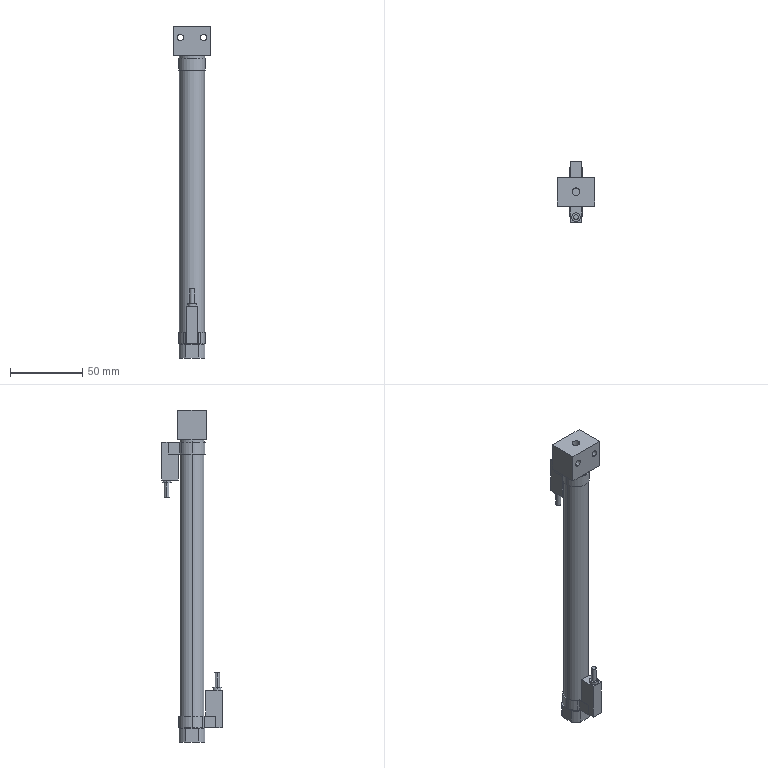Part | NX | features BREP 1 | 1 solid | 96 faces | box 26 x 41.8 x 230 mm | volume 61540 mm3 | plane 52 | cylinder 40 | cone 4 | commonest cylinder face diameters 18.6 x8 17.4 x6 3.4 x4 4.13 x4 4.5 x4 6 x4